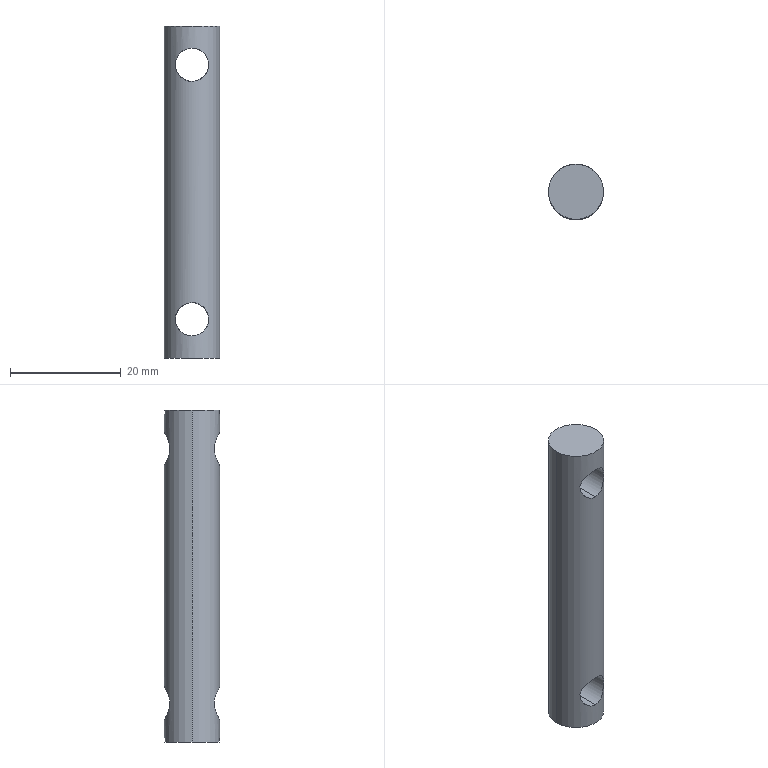Part | SolidWorks | features Extrusion 1, ICE 1 | 1 solid | 8 faces | box 10 x 10 x 60 mm | volume 4174 mm3 | cylinder 6 | plane 2 | commonest cylinder face diameters 6 x4 10 x2
STEP:
#1=CARTESIAN_POINT('',(0.,-5.,4.));
#2=VERTEX_POINT('',#1);
#3=CARTESIAN_POINT('',(0.,-5.,10.));
#4=VERTEX_POINT('',#3);
#5=CARTESIAN_POINT('',(0.,-5.,4.));
#6=CARTESIAN_POINT('',(-0.2026,-5.,4.));
#7=CARTESIAN_POINT('',(-0.4018,-4.988,4.02));
#8=CARTESIAN_POINT('',(-0.7938,-4.941,4.1));
#9=CARTESIAN_POINT('',(-0.9867,-4.905,4.16));
#10=CARTESIAN_POINT('',(-1.348,-4.818,4.313));
#11=CARTESIAN_POINT('',(-1.521,-4.766,4.407));
#12=CARTESIAN_POINT('',(-1.843,-4.651,4.625));
#13=CARTESIAN_POINT('',(-1.99,-4.589,4.747));
#14=CARTESIAN_POINT('',(-2.26,-4.463,5.018));
#15=CARTESIAN_POINT('',(-2.383,-4.397,5.167));
#16=CARTESIAN_POINT('',(-2.596,-4.275,5.485));
#17=CARTESIAN_POINT('',(-2.688,-4.217,5.653));
#18=CARTESIAN_POINT('',(-2.84,-4.116,6.014));
#19=CARTESIAN_POINT('',(-2.899,-4.074,6.204));
#20=CARTESIAN_POINT('',(-2.979,-4.016,6.594));
#21=CARTESIAN_POINT('',(-3.,-4.,6.798));
#22=CARTESIAN_POINT('',(-3.,-4.,7.201));
#23=CARTESIAN_POINT('',(-2.98,-4.015,7.4));
#24=CARTESIAN_POINT('',(-2.9,-4.073,7.794));
#25=CARTESIAN_POINT('',(-2.841,-4.115,7.983));
#26=CARTESIAN_POINT('',(-2.689,-4.216,8.344));
#27=CARTESIAN_POINT('',(-2.596,-4.275,8.516));
#28=CARTESIAN_POINT('',(-2.382,-4.398,8.834));
#29=CARTESIAN_POINT('',(-2.26,-4.462,8.982));
#30=CARTESIAN_POINT('',(-1.988,-4.59,9.255));
#31=CARTESIAN_POINT('',(-1.84,-4.652,9.377));
#32=CARTESIAN_POINT('',(-1.522,-4.766,9.592));
#33=CARTESIAN_POINT('',(-1.349,-4.818,9.687));
#34=CARTESIAN_POINT('',(-0.9853,-4.906,9.84));
#35=CARTESIAN_POINT('',(-0.797,-4.94,9.899));
#36=CARTESIAN_POINT('',(-0.4074,-4.987,9.979));
#37=CARTESIAN_POINT('',(-0.2033,-5.,10.));
#38=CARTESIAN_POINT('',(0.,-5.,10.));
#39=B_SPLINE_CURVE_WITH_KNOTS('',3,(#5,#6,#7,#8,#9,#10,#11,#12,#13,#14,#15,#16,#17,#18,#19,#20,#21,#22,#23,#24,#25,#26,#27,#28,#29,#30,#31,#32,#33,#34,#35,#36,#37,#38),.UNSPECIFIED.,.F.,.F.,(4,2,2,2,2,2,2,2,2,2,2,2,2,2,2,2,4),(0.009625,0.01023,0.01083,0.01143,0.01203,0.01263,0.01323,0.01383,0.01443,0.01503,0.01563,0.01623,0.01683,0.01743,0.01803,0.01863,0.01923),.UNSPECIFIED.);
#40=EDGE_CURVE('',#2,#4,#39,.T.);
#41=ORIENTED_EDGE('',*,*,#40,.F.);
#42=CARTESIAN_POINT('',(0.,5.,4.));
#43=VERTEX_POINT('',#42);
#44=CARTESIAN_POINT('',(0.,-5.,4.));
#45=DIRECTION('',(0.,1.,0.));
#46=VECTOR('',#45,1000.);
#47=LINE('',#44,#46);
#48=EDGE_CURVE('',#2,#43,#47,.T.);
#49=ORIENTED_EDGE('',*,*,#48,.T.);
#50=CARTESIAN_POINT('',(0.,5.,10.));
#51=VERTEX_POINT('',#50);
#52=CARTESIAN_POINT('',(0.,5.,10.));
#53=CARTESIAN_POINT('',(-0.2037,5.,10.));
#54=CARTESIAN_POINT('',(-0.4031,4.988,9.979));
#55=CARTESIAN_POINT('',(-0.794,4.94,9.9));
#56=CARTESIAN_POINT('',(-0.9871,4.905,9.84));
#57=CARTESIAN_POINT('',(-1.53,4.775,9.61));
#58=CARTESIAN_POINT('',(-1.856,4.652,9.388));
#59=CARTESIAN_POINT('',(-2.26,4.463,8.982));
#60=CARTESIAN_POINT('',(-2.383,4.397,8.833));
#61=CARTESIAN_POINT('',(-2.597,4.275,8.514));
#62=CARTESIAN_POINT('',(-2.688,4.217,8.346));
#63=CARTESIAN_POINT('',(-2.839,4.117,7.988));
#64=CARTESIAN_POINT('',(-2.899,4.074,7.796));
#65=CARTESIAN_POINT('',(-2.979,4.016,7.405));
#66=CARTESIAN_POINT('',(-3.,4.,7.204));
#67=CARTESIAN_POINT('',(-3.,4.,6.798));
#68=CARTESIAN_POINT('',(-2.98,4.015,6.598));
#69=CARTESIAN_POINT('',(-2.9,4.073,6.207));
#70=CARTESIAN_POINT('',(-2.841,4.116,6.015));
#71=CARTESIAN_POINT('',(-2.689,4.216,5.656));
#72=CARTESIAN_POINT('',(-2.596,4.275,5.484));
#73=CARTESIAN_POINT('',(-2.381,4.399,5.164));
#74=CARTESIAN_POINT('',(-2.259,4.463,5.017));
#75=CARTESIAN_POINT('',(-1.988,4.59,4.745));
#76=CARTESIAN_POINT('',(-1.839,4.653,4.622));
#77=CARTESIAN_POINT('',(-1.52,4.766,4.406));
#78=CARTESIAN_POINT('',(-1.35,4.818,4.314));
#79=CARTESIAN_POINT('',(-0.8028,4.949,4.082));
#80=CARTESIAN_POINT('',(-0.406,5.,4.));
#81=CARTESIAN_POINT('',(0.,5.,4.));
#82=B_SPLINE_CURVE_WITH_KNOTS('',3,(#52,#53,#54,#55,#56,#57,#58,#59,#60,#61,#62,#63,#64,#65,#66,#67,#68,#69,#70,#71,#72,#73,#74,#75,#76,#77,#78,#79,#80,#81),.UNSPECIFIED.,.F.,.F.,(4,2,2,2,2,2,2,2,2,2,2,2,2,2,4),(0.,0.0006015,0.001203,0.002406,0.003008,0.003609,0.004211,0.004812,0.005414,0.006015,0.006617,0.007219,0.00782,0.008422,0.009625),.UNSPECIFIED.);
#83=EDGE_CURVE('',#51,#43,#82,.T.);
#84=ORIENTED_EDGE('',*,*,#83,.F.);
#85=CARTESIAN_POINT('',(0.,-5.,10.));
#86=DIRECTION('',(0.,1.,0.));
#87=VECTOR('',#86,1000.);
#88=LINE('',#85,#87);
#89=EDGE_CURVE('',#4,#51,#88,.T.);
#90=ORIENTED_EDGE('',*,*,#89,.F.);
#91=EDGE_LOOP('',(#41,#49,#84,#90));
#92=FACE_OUTER_BOUND('',#91,.T.);
#93=CARTESIAN_POINT('',(0.,-5.,7.));
#94=DIRECTION('',(0.,1.,0.));
#95=DIRECTION('',(0.,0.,1.));
#96=AXIS2_PLACEMENT_3D('',#93,#94,#95);
#97=CYLINDRICAL_SURFACE('',#96,3.);
#98=ADVANCED_FACE('',(#92),#97,.F.);
#99=CARTESIAN_POINT('',(0.,-5.,50.));
#100=VERTEX_POINT('',#99);
#101=CARTESIAN_POINT('',(0.,-5.,56.));
#102=VERTEX_POINT('',#101);
#103=CARTESIAN_POINT('',(0.,-5.,50.));
#104=CARTESIAN_POINT('',(-0.2026,-5.,50.));
#105=CARTESIAN_POINT('',(-0.4018,-4.988,50.02));
#106=CARTESIAN_POINT('',(-0.7938,-4.941,50.1));
#107=CARTESIAN_POINT('',(-0.9867,-4.905,50.16));
#108=CARTESIAN_POINT('',(-1.348,-4.818,50.313));
#109=CARTESIAN_POINT('',(-1.521,-4.766,50.407));
#110=CARTESIAN_POINT('',(-1.843,-4.651,50.625));
#111=CARTESIAN_POINT('',(-1.99,-4.589,50.747));
#112=CARTESIAN_POINT('',(-2.26,-4.463,51.018));
#113=CARTESIAN_POINT('',(-2.383,-4.397,51.167));
#114=CARTESIAN_POINT('',(-2.596,-4.275,51.485));
#115=CARTESIAN_POINT('',(-2.688,-4.217,51.653));
#116=CARTESIAN_POINT('',(-2.84,-4.116,52.014));
#117=CARTESIAN_POINT('',(-2.899,-4.074,52.204));
#118=CARTESIAN_POINT('',(-2.979,-4.016,52.594));
#119=CARTESIAN_POINT('',(-3.,-4.,52.798));
#120=CARTESIAN_POINT('',(-3.,-4.,53.201));
#121=CARTESIAN_POINT('',(-2.98,-4.015,53.4));
#122=CARTESIAN_POINT('',(-2.9,-4.073,53.794));
#123=CARTESIAN_POINT('',(-2.841,-4.115,53.983));
#124=CARTESIAN_POINT('',(-2.689,-4.216,54.344));
#125=CARTESIAN_POINT('',(-2.596,-4.275,54.516));
#126=CARTESIAN_POINT('',(-2.382,-4.398,54.834));
#127=CARTESIAN_POINT('',(-2.26,-4.462,54.982));
#128=CARTESIAN_POINT('',(-1.988,-4.59,55.255));
#129=CARTESIAN_POINT('',(-1.84,-4.652,55.377));
#130=CARTESIAN_POINT('',(-1.522,-4.766,55.592));
#131=CARTESIAN_POINT('',(-1.349,-4.818,55.687));
#132=CARTESIAN_POINT('',(-0.9853,-4.906,55.84));
#133=CARTESIAN_POINT('',(-0.797,-4.94,55.899));
#134=CARTESIAN_POINT('',(-0.4074,-4.987,55.979));
#135=CARTESIAN_POINT('',(-0.2033,-5.,56.));
#136=CARTESIAN_POINT('',(0.,-5.,56.));
#137=B_SPLINE_CURVE_WITH_KNOTS('',3,(#103,#104,#105,#106,#107,#108,#109,#110,#111,#112,#113,#114,#115,#116,#117,#118,#119,#120,#121,#122,#123,#124,#125,#126,#127,#128,#129,#130,#131,#132,#133,#134,#135,#136),.UNSPECIFIED.,.F.,.F.,(4,2,2,2,2,2,2,2,2,2,2,2,2,2,2,2,4),(0.009625,0.01023,0.01083,0.01143,0.01203,0.01263,0.01323,0.01383,0.01443,0.01503,0.01563,0.01623,0.01683,0.01743,0.01803,0.01863,0.01923),.UNSPECIFIED.);
#138=EDGE_CURVE('',#100,#102,#137,.T.);
#139=ORIENTED_EDGE('',*,*,#138,.F.);
#140=CARTESIAN_POINT('',(0.,5.,50.));
#141=VERTEX_POINT('',#140);
#142=CARTESIAN_POINT('',(0.,-5.,50.));
#143=DIRECTION('',(0.,1.,0.));
#144=VECTOR('',#143,1000.);
#145=LINE('',#142,#144);
#146=EDGE_CURVE('',#100,#141,#145,.T.);
#147=ORIENTED_EDGE('',*,*,#146,.T.);
#148=CARTESIAN_POINT('',(0.,5.,56.));
#149=VERTEX_POINT('',#148);
#150=CARTESIAN_POINT('',(0.,5.,56.));
#151=CARTESIAN_POINT('',(-0.2037,5.,56.));
#152=CARTESIAN_POINT('',(-0.4031,4.988,55.979));
#153=CARTESIAN_POINT('',(-0.794,4.94,55.9));
#154=CARTESIAN_POINT('',(-0.9871,4.905,55.84));
#155=CARTESIAN_POINT('',(-1.53,4.775,55.61));
#156=CARTESIAN_POINT('',(-1.856,4.652,55.388));
#157=CARTESIAN_POINT('',(-2.26,4.463,54.982));
#158=CARTESIAN_POINT('',(-2.383,4.397,54.833));
#159=CARTESIAN_POINT('',(-2.597,4.275,54.514));
#160=CARTESIAN_POINT('',(-2.688,4.217,54.346));
#161=CARTESIAN_POINT('',(-2.839,4.117,53.988));
#162=CARTESIAN_POINT('',(-2.899,4.074,53.796));
#163=CARTESIAN_POINT('',(-2.979,4.016,53.405));
#164=CARTESIAN_POINT('',(-3.,4.,53.204));
#165=CARTESIAN_POINT('',(-3.,4.,52.798));
#166=CARTESIAN_POINT('',(-2.98,4.015,52.598));
#167=CARTESIAN_POINT('',(-2.9,4.073,52.207));
#168=CARTESIAN_POINT('',(-2.841,4.116,52.015));
#169=CARTESIAN_POINT('',(-2.689,4.216,51.656));
#170=CARTESIAN_POINT('',(-2.596,4.275,51.484));
#171=CARTESIAN_POINT('',(-2.381,4.399,51.164));
#172=CARTESIAN_POINT('',(-2.259,4.463,51.017));
#173=CARTESIAN_POINT('',(-1.988,4.59,50.745));
#174=CARTESIAN_POINT('',(-1.839,4.653,50.622));
#175=CARTESIAN_POINT('',(-1.52,4.766,50.406));
#176=CARTESIAN_POINT('',(-1.35,4.818,50.314));
#177=CARTESIAN_POINT('',(-0.8028,4.949,50.082));
#178=CARTESIAN_POINT('',(-0.406,5.,50.));
#179=CARTESIAN_POINT('',(0.,5.,50.));
#180=B_SPLINE_CURVE_WITH_KNOTS('',3,(#150,#151,#152,#153,#154,#155,#156,#157,#158,#159,#160,#161,#162,#163,#164,#165,#166,#167,#168,#169,#170,#171,#172,#173,#174,#175,#176,#177,#178,#179),.UNSPECIFIED.,.F.,.F.,(4,2,2,2,2,2,2,2,2,2,2,2,2,2,4),(0.,0.0006015,0.001203,0.002406,0.003008,0.003609,0.004211,0.004812,0.005414,0.006015,0.006617,0.007219,0.00782,0.008422,0.009625),.UNSPECIFIED.);
#181=EDGE_CURVE('',#149,#141,#180,.T.);
#182=ORIENTED_EDGE('',*,*,#181,.F.);
#183=CARTESIAN_POINT('',(0.,-5.,56.));
#184=DIRECTION('',(0.,1.,0.));
#185=VECTOR('',#184,1000.);
#186=LINE('',#183,#185);
#187=EDGE_CURVE('',#102,#149,#186,.T.);
#188=ORIENTED_EDGE('',*,*,#187,.F.);
#189=EDGE_LOOP('',(#139,#147,#182,#188));
#190=FACE_OUTER_BOUND('',#189,.T.);
#191=CARTESIAN_POINT('',(0.,-5.,53.));
#192=DIRECTION('',(0.,1.,0.));
#193=DIRECTION('',(0.,0.,1.));
#194=AXIS2_PLACEMENT_3D('',#191,#192,#193);
#195=CYLINDRICAL_SURFACE('',#194,3.);
#196=ADVANCED_FACE('',(#190),#195,.F.);
#197=ORIENTED_EDGE('',*,*,#181,.T.);
#198=CARTESIAN_POINT('',(0.,5.,50.));
#199=CARTESIAN_POINT('',(0.2026,5.,50.));
#200=CARTESIAN_POINT('',(0.4018,4.988,50.02));
#201=CARTESIAN_POINT('',(0.7938,4.941,50.1));
#202=CARTESIAN_POINT('',(0.9867,4.905,50.16));
#203=CARTESIAN_POINT('',(1.348,4.818,50.313));
#204=CARTESIAN_POINT('',(1.521,4.766,50.407));
#205=CARTESIAN_POINT('',(1.843,4.651,50.625));
#206=CARTESIAN_POINT('',(1.99,4.589,50.747));
#207=CARTESIAN_POINT('',(2.26,4.463,51.018));
#208=CARTESIAN_POINT('',(2.383,4.397,51.167));
#209=CARTESIAN_POINT('',(2.596,4.275,51.485));
#210=CARTESIAN_POINT('',(2.688,4.217,51.653));
#211=CARTESIAN_POINT('',(2.84,4.116,52.014));
#212=CARTESIAN_POINT('',(2.899,4.074,52.204));
#213=CARTESIAN_POINT('',(2.979,4.016,52.594));
#214=CARTESIAN_POINT('',(3.,4.,52.798));
#215=CARTESIAN_POINT('',(3.,4.,53.201));
#216=CARTESIAN_POINT('',(2.98,4.015,53.4));
#217=CARTESIAN_POINT('',(2.9,4.073,53.794));
#218=CARTESIAN_POINT('',(2.841,4.115,53.983));
#219=CARTESIAN_POINT('',(2.689,4.216,54.344));
#220=CARTESIAN_POINT('',(2.596,4.275,54.516));
#221=CARTESIAN_POINT('',(2.382,4.398,54.834));
#222=CARTESIAN_POINT('',(2.26,4.462,54.982));
#223=CARTESIAN_POINT('',(1.988,4.59,55.255));
#224=CARTESIAN_POINT('',(1.84,4.652,55.377));
#225=CARTESIAN_POINT('',(1.522,4.766,55.592));
#226=CARTESIAN_POINT('',(1.349,4.818,55.687));
#227=CARTESIAN_POINT('',(0.9853,4.906,55.84));
#228=CARTESIAN_POINT('',(0.797,4.94,55.899));
#229=CARTESIAN_POINT('',(0.4074,4.987,55.979));
#230=CARTESIAN_POINT('',(0.2033,5.,56.));
#231=CARTESIAN_POINT('',(0.,5.,56.));
#232=B_SPLINE_CURVE_WITH_KNOTS('',3,(#198,#199,#200,#201,#202,#203,#204,#205,#206,#207,#208,#209,#210,#211,#212,#213,#214,#215,#216,#217,#218,#219,#220,#221,#222,#223,#224,#225,#226,#227,#228,#229,#230,#231),.UNSPECIFIED.,.F.,.F.,(4,2,2,2,2,2,2,2,2,2,2,2,2,2,2,2,4),(0.009625,0.01023,0.01083,0.01143,0.01203,0.01263,0.01323,0.01383,0.01443,0.01503,0.01563,0.01623,0.01683,0.01743,0.01803,0.01863,0.01923),.UNSPECIFIED.);
#233=EDGE_CURVE('',#141,#149,#232,.T.);
#234=ORIENTED_EDGE('',*,*,#233,.T.);
#235=EDGE_LOOP('',(#197,#234));
#236=FACE_BOUND('',#235,.T.);
#237=ORIENTED_EDGE('',*,*,#83,.T.);
#238=CARTESIAN_POINT('',(0.,5.,4.));
#239=CARTESIAN_POINT('',(0.2026,5.,4.));
#240=CARTESIAN_POINT('',(0.4018,4.988,4.02));
#241=CARTESIAN_POINT('',(0.7938,4.941,4.1));
#242=CARTESIAN_POINT('',(0.9867,4.905,4.16));
#243=CARTESIAN_POINT('',(1.348,4.818,4.313));
#244=CARTESIAN_POINT('',(1.521,4.766,4.407));
#245=CARTESIAN_POINT('',(1.843,4.651,4.625));
#246=CARTESIAN_POINT('',(1.99,4.589,4.747));
#247=CARTESIAN_POINT('',(2.26,4.463,5.018));
#248=CARTESIAN_POINT('',(2.383,4.397,5.167));
#249=CARTESIAN_POINT('',(2.596,4.275,5.485));
#250=CARTESIAN_POINT('',(2.688,4.217,5.653));
#251=CARTESIAN_POINT('',(2.84,4.116,6.014));
#252=CARTESIAN_POINT('',(2.899,4.074,6.204));
#253=CARTESIAN_POINT('',(2.979,4.016,6.594));
#254=CARTESIAN_POINT('',(3.,4.,6.798));
#255=CARTESIAN_POINT('',(3.,4.,7.201));
#256=CARTESIAN_POINT('',(2.98,4.015,7.4));
#257=CARTESIAN_POINT('',(2.9,4.073,7.794));
#258=CARTESIAN_POINT('',(2.841,4.115,7.983));
#259=CARTESIAN_POINT('',(2.689,4.216,8.344));
#260=CARTESIAN_POINT('',(2.596,4.275,8.516));
#261=CARTESIAN_POINT('',(2.382,4.398,8.834));
#262=CARTESIAN_POINT('',(2.26,4.462,8.982));
#263=CARTESIAN_POINT('',(1.988,4.59,9.255));
#264=CARTESIAN_POINT('',(1.84,4.652,9.377));
#265=CARTESIAN_POINT('',(1.522,4.766,9.592));
#266=CARTESIAN_POINT('',(1.349,4.818,9.687));
#267=CARTESIAN_POINT('',(0.9853,4.906,9.84));
#268=CARTESIAN_POINT('',(0.797,4.94,9.899));
#269=CARTESIAN_POINT('',(0.4074,4.987,9.979));
#270=CARTESIAN_POINT('',(0.2033,5.,10.));
#271=CARTESIAN_POINT('',(0.,5.,10.));
#272=B_SPLINE_CURVE_WITH_KNOTS('',3,(#238,#239,#240,#241,#242,#243,#244,#245,#246,#247,#248,#249,#250,#251,#252,#253,#254,#255,#256,#257,#258,#259,#260,#261,#262,#263,#264,#265,#266,#267,#268,#269,#270,#271),.UNSPECIFIED.,.F.,.F.,(4,2,2,2,2,2,2,2,2,2,2,2,2,2,2,2,4),(0.009625,0.01023,0.01083,0.01143,0.01203,0.01263,0.01323,0.01383,0.01443,0.01503,0.01563,0.01623,0.01683,0.01743,0.01803,0.01863,0.01923),.UNSPECIFIED.);
#273=EDGE_CURVE('',#43,#51,#272,.T.);
#274=ORIENTED_EDGE('',*,*,#273,.T.);
#275=EDGE_LOOP('',(#237,#274));
#276=FACE_BOUND('',#275,.T.);
#277=CARTESIAN_POINT('',(5.,0.,60.));
#278=VERTEX_POINT('',#277);
#279=CARTESIAN_POINT('',(-5.,0.,60.));
#280=VERTEX_POINT('',#279);
#281=CARTESIAN_POINT('',(0.,0.,60.));
#282=DIRECTION('',(0.,0.,1.));
#283=DIRECTION('',(1.,0.,0.));
#284=AXIS2_PLACEMENT_3D('',#281,#282,#283);
#285=CIRCLE('',#284,5.);
#286=EDGE_CURVE('',#278,#280,#285,.T.);
#287=ORIENTED_EDGE('',*,*,#286,.F.);
#288=CARTESIAN_POINT('',(5.,0.,0.));
#289=VERTEX_POINT('',#288);
#290=CARTESIAN_POINT('',(5.,0.,60.));
#291=DIRECTION('',(0.,0.,-1.));
#292=VECTOR('',#291,1000.);
#293=LINE('',#290,#292);
#294=EDGE_CURVE('',#278,#289,#293,.T.);
#295=ORIENTED_EDGE('',*,*,#294,.T.);
#296=CARTESIAN_POINT('',(-5.,0.,0.));
#297=VERTEX_POINT('',#296);
#298=CARTESIAN_POINT('',(0.,0.,0.));
#299=DIRECTION('',(0.,0.,1.));
#300=DIRECTION('',(1.,0.,0.));
#301=AXIS2_PLACEMENT_3D('',#298,#299,#300);
#302=CIRCLE('',#301,5.);
#303=EDGE_CURVE('',#289,#297,#302,.T.);
#304=ORIENTED_EDGE('',*,*,#303,.T.);
#305=CARTESIAN_POINT('',(-5.,0.,60.));
#306=DIRECTION('',(0.,0.,-1.));
#307=VECTOR('',#306,1000.);
#308=LINE('',#305,#307);
#309=EDGE_CURVE('',#280,#297,#308,.T.);
#310=ORIENTED_EDGE('',*,*,#309,.F.);
#311=EDGE_LOOP('',(#287,#295,#304,#310));
#312=FACE_OUTER_BOUND('',#311,.T.);
#313=CARTESIAN_POINT('',(0.,0.,60.));
#314=DIRECTION('',(0.,0.,-1.));
#315=DIRECTION('',(-1.,0.,0.));
#316=AXIS2_PLACEMENT_3D('',#313,#314,#315);
#317=CYLINDRICAL_SURFACE('',#316,5.);
#318=ADVANCED_FACE('',(#236,#276,#312),#317,.T.);
#319=ORIENTED_EDGE('',*,*,#294,.F.);
#320=CARTESIAN_POINT('',(0.,0.,60.));
#321=DIRECTION('',(0.,0.,1.));
#322=DIRECTION('',(1.,0.,0.));
#323=AXIS2_PLACEMENT_3D('',#320,#321,#322);
#324=CIRCLE('',#323,5.);
#325=EDGE_CURVE('',#280,#278,#324,.T.);
#326=ORIENTED_EDGE('',*,*,#325,.F.);
#327=ORIENTED_EDGE('',*,*,#309,.T.);
#328=CARTESIAN_POINT('',(0.,0.,0.));
#329=DIRECTION('',(0.,0.,1.));
#330=DIRECTION('',(1.,0.,0.));
#331=AXIS2_PLACEMENT_3D('',#328,#329,#330);
#332=CIRCLE('',#331,5.);
#333=EDGE_CURVE('',#297,#289,#332,.T.);
#334=ORIENTED_EDGE('',*,*,#333,.T.);
#335=EDGE_LOOP('',(#319,#326,#327,#334));
#336=FACE_OUTER_BOUND('',#335,.T.);
#337=CARTESIAN_POINT('',(0.,-5.,10.));
#338=CARTESIAN_POINT('',(0.2037,-5.,10.));
#339=CARTESIAN_POINT('',(0.4031,-4.988,9.979));
#340=CARTESIAN_POINT('',(0.794,-4.94,9.9));
#341=CARTESIAN_POINT('',(0.9871,-4.905,9.84));
#342=CARTESIAN_POINT('',(1.53,-4.775,9.61));
#343=CARTESIAN_POINT('',(1.856,-4.652,9.388));
#344=CARTESIAN_POINT('',(2.26,-4.463,8.982));
#345=CARTESIAN_POINT('',(2.383,-4.397,8.833));
#346=CARTESIAN_POINT('',(2.597,-4.275,8.514));
#347=CARTESIAN_POINT('',(2.688,-4.217,8.346));
#348=CARTESIAN_POINT('',(2.839,-4.117,7.988));
#349=CARTESIAN_POINT('',(2.899,-4.074,7.796));
#350=CARTESIAN_POINT('',(2.979,-4.016,7.405));
#351=CARTESIAN_POINT('',(3.,-4.,7.204));
#352=CARTESIAN_POINT('',(3.,-4.,6.798));
#353=CARTESIAN_POINT('',(2.98,-4.015,6.598));
#354=CARTESIAN_POINT('',(2.9,-4.073,6.207));
#355=CARTESIAN_POINT('',(2.841,-4.116,6.015));
#356=CARTESIAN_POINT('',(2.689,-4.216,5.656));
#357=CARTESIAN_POINT('',(2.596,-4.275,5.484));
#358=CARTESIAN_POINT('',(2.381,-4.399,5.164));
#359=CARTESIAN_POINT('',(2.259,-4.463,5.017));
#360=CARTESIAN_POINT('',(1.988,-4.59,4.745));
#361=CARTESIAN_POINT('',(1.839,-4.653,4.622));
#362=CARTESIAN_POINT('',(1.52,-4.766,4.406));
#363=CARTESIAN_POINT('',(1.35,-4.818,4.314));
#364=CARTESIAN_POINT('',(0.8028,-4.949,4.082));
#365=CARTESIAN_POINT('',(0.406,-5.,4.));
#366=CARTESIAN_POINT('',(0.,-5.,4.));
#367=B_SPLINE_CURVE_WITH_KNOTS('',3,(#337,#338,#339,#340,#341,#342,#343,#344,#345,#346,#347,#348,#349,#350,#351,#352,#353,#354,#355,#356,#357,#358,#359,#360,#361,#362,#363,#364,#365,#366),.UNSPECIFIED.,.F.,.F.,(4,2,2,2,2,2,2,2,2,2,2,2,2,2,4),(0.,0.0006015,0.001203,0.002406,0.003008,0.003609,0.004211,0.004812,0.005414,0.006015,0.006617,0.007219,0.00782,0.008422,0.009625),.UNSPECIFIED.);
#368=EDGE_CURVE('',#4,#2,#367,.T.);
#369=ORIENTED_EDGE('',*,*,#368,.T.);
#370=ORIENTED_EDGE('',*,*,#40,.T.);
#371=EDGE_LOOP('',(#369,#370));
#372=FACE_BOUND('',#371,.T.);
#373=CARTESIAN_POINT('',(0.,-5.,56.));
#374=CARTESIAN_POINT('',(0.2037,-5.,56.));
#375=CARTESIAN_POINT('',(0.4031,-4.988,55.979));
#376=CARTESIAN_POINT('',(0.794,-4.94,55.9));
#377=CARTESIAN_POINT('',(0.9871,-4.905,55.84));
#378=CARTESIAN_POINT('',(1.53,-4.775,55.61));
#379=CARTESIAN_POINT('',(1.856,-4.652,55.388));
#380=CARTESIAN_POINT('',(2.26,-4.463,54.982));
#381=CARTESIAN_POINT('',(2.383,-4.397,54.833));
#382=CARTESIAN_POINT('',(2.597,-4.275,54.514));
#383=CARTESIAN_POINT('',(2.688,-4.217,54.346));
#384=CARTESIAN_POINT('',(2.839,-4.117,53.988));
#385=CARTESIAN_POINT('',(2.899,-4.074,53.796));
#386=CARTESIAN_POINT('',(2.979,-4.016,53.405));
#387=CARTESIAN_POINT('',(3.,-4.,53.204));
#388=CARTESIAN_POINT('',(3.,-4.,52.798));
#389=CARTESIAN_POINT('',(2.98,-4.015,52.598));
#390=CARTESIAN_POINT('',(2.9,-4.073,52.207));
#391=CARTESIAN_POINT('',(2.841,-4.116,52.015));
#392=CARTESIAN_POINT('',(2.689,-4.216,51.656));
#393=CARTESIAN_POINT('',(2.596,-4.275,51.484));
#394=CARTESIAN_POINT('',(2.381,-4.399,51.164));
#395=CARTESIAN_POINT('',(2.259,-4.463,51.017));
#396=CARTESIAN_POINT('',(1.988,-4.59,50.745));
#397=CARTESIAN_POINT('',(1.839,-4.653,50.622));
#398=CARTESIAN_POINT('',(1.52,-4.766,50.406));
#399=CARTESIAN_POINT('',(1.35,-4.818,50.314));
#400=CARTESIAN_POINT('',(0.8028,-4.949,50.082));
#401=CARTESIAN_POINT('',(0.406,-5.,50.));
#402=CARTESIAN_POINT('',(0.,-5.,50.));
#403=B_SPLINE_CURVE_WITH_KNOTS('',3,(#373,#374,#375,#376,#377,#378,#379,#380,#381,#382,#383,#384,#385,#386,#387,#388,#389,#390,#391,#392,#393,#394,#395,#396,#397,#398,#399,#400,#401,#402),.UNSPECIFIED.,.F.,.F.,(4,2,2,2,2,2,2,2,2,2,2,2,2,2,4),(0.,0.0006015,0.001203,0.002406,0.003008,0.003609,0.004211,0.004812,0.005414,0.006015,0.006617,0.007219,0.00782,0.008422,0.009625),.UNSPECIFIED.);
#404=EDGE_CURVE('',#102,#100,#403,.T.);
#405=ORIENTED_EDGE('',*,*,#404,.T.);
#406=ORIENTED_EDGE('',*,*,#138,.T.);
#407=EDGE_LOOP('',(#405,#406));
#408=FACE_BOUND('',#407,.T.);
#409=CARTESIAN_POINT('',(0.,0.,60.));
#410=DIRECTION('',(0.,0.,-1.));
#411=DIRECTION('',(-1.,0.,0.));
#412=AXIS2_PLACEMENT_3D('',#409,#410,#411);
#413=CYLINDRICAL_SURFACE('',#412,5.);
#414=ADVANCED_FACE('',(#336,#372,#408),#413,.T.);
#415=ORIENTED_EDGE('',*,*,#325,.T.);
#416=ORIENTED_EDGE('',*,*,#286,.T.);
#417=EDGE_LOOP('',(#415,#416));
#418=FACE_OUTER_BOUND('',#417,.T.);
#419=CARTESIAN_POINT('',(0.,0.,60.));
#420=DIRECTION('',(0.,0.,1.));
#421=DIRECTION('',(1.,0.,0.));
#422=AXIS2_PLACEMENT_3D('',#419,#420,#421);
#423=PLANE('',#422);
#424=ADVANCED_FACE('',(#418),#423,.T.);
#425=ORIENTED_EDGE('',*,*,#333,.F.);
#426=ORIENTED_EDGE('',*,*,#303,.F.);
#427=EDGE_LOOP('',(#425,#426));
#428=FACE_OUTER_BOUND('',#427,.T.);
#429=CARTESIAN_POINT('',(0.,0.,0.));
#430=DIRECTION('',(0.,0.,1.));
#431=DIRECTION('',(1.,0.,0.));
#432=AXIS2_PLACEMENT_3D('',#429,#430,#431);
#433=PLANE('',#432);
#434=ADVANCED_FACE('',(#428),#433,.F.);
#435=ORIENTED_EDGE('',*,*,#146,.F.);
#436=ORIENTED_EDGE('',*,*,#404,.F.);
#437=ORIENTED_EDGE('',*,*,#187,.T.);
#438=ORIENTED_EDGE('',*,*,#233,.F.);
#439=EDGE_LOOP('',(#435,#436,#437,#438));
#440=FACE_OUTER_BOUND('',#439,.T.);
#441=CARTESIAN_POINT('',(0.,-5.,53.));
#442=DIRECTION('',(0.,1.,0.));
#443=DIRECTION('',(0.,0.,1.));
#444=AXIS2_PLACEMENT_3D('',#441,#442,#443);
#445=CYLINDRICAL_SURFACE('',#444,3.);
#446=ADVANCED_FACE('',(#440),#445,.F.);
#447=ORIENTED_EDGE('',*,*,#48,.F.);
#448=ORIENTED_EDGE('',*,*,#368,.F.);
#449=ORIENTED_EDGE('',*,*,#89,.T.);
#450=ORIENTED_EDGE('',*,*,#273,.F.);
#451=EDGE_LOOP('',(#447,#448,#449,#450));
#452=FACE_OUTER_BOUND('',#451,.T.);
#453=CARTESIAN_POINT('',(0.,-5.,7.));
#454=DIRECTION('',(0.,1.,0.));
#455=DIRECTION('',(0.,0.,1.));
#456=AXIS2_PLACEMENT_3D('',#453,#454,#455);
#457=CYLINDRICAL_SURFACE('',#456,3.);
#458=ADVANCED_FACE('',(#452),#457,.F.);
#459=CLOSED_SHELL('',(#98,#196,#318,#414,#424,#434,#446,#458));
#460=MANIFOLD_SOLID_BREP('',#459);
#461=CARTESIAN_POINT('',(0.,0.,0.));
#462=DIRECTION('',(0.,0.,1.));
#463=DIRECTION('',(1.,0.,0.));
#464=AXIS2_PLACEMENT_3D('',#461,#462,#463);
#465=(LENGTH_UNIT()NAMED_UNIT(*)SI_UNIT(.MILLI.,.METRE.));
#466=UNCERTAINTY_MEASURE_WITH_UNIT(LENGTH_MEASURE(0.00001),#465,'','');
#467=(NAMED_UNIT(*)PLANE_ANGLE_UNIT()SI_UNIT($,.RADIAN.));
#468=(NAMED_UNIT(*)SI_UNIT($,.STERADIAN.)SOLID_ANGLE_UNIT());
#469=(GEOMETRIC_REPRESENTATION_CONTEXT(3)GLOBAL_UNCERTAINTY_ASSIGNED_CONTEXT((#466))GLOBAL_UNIT_ASSIGNED_CONTEXT((#465,#467,#468))REPRESENTATION_CONTEXT('',''));
#470=ADVANCED_BREP_SHAPE_REPRESENTATION('',(#460,#464),#469);